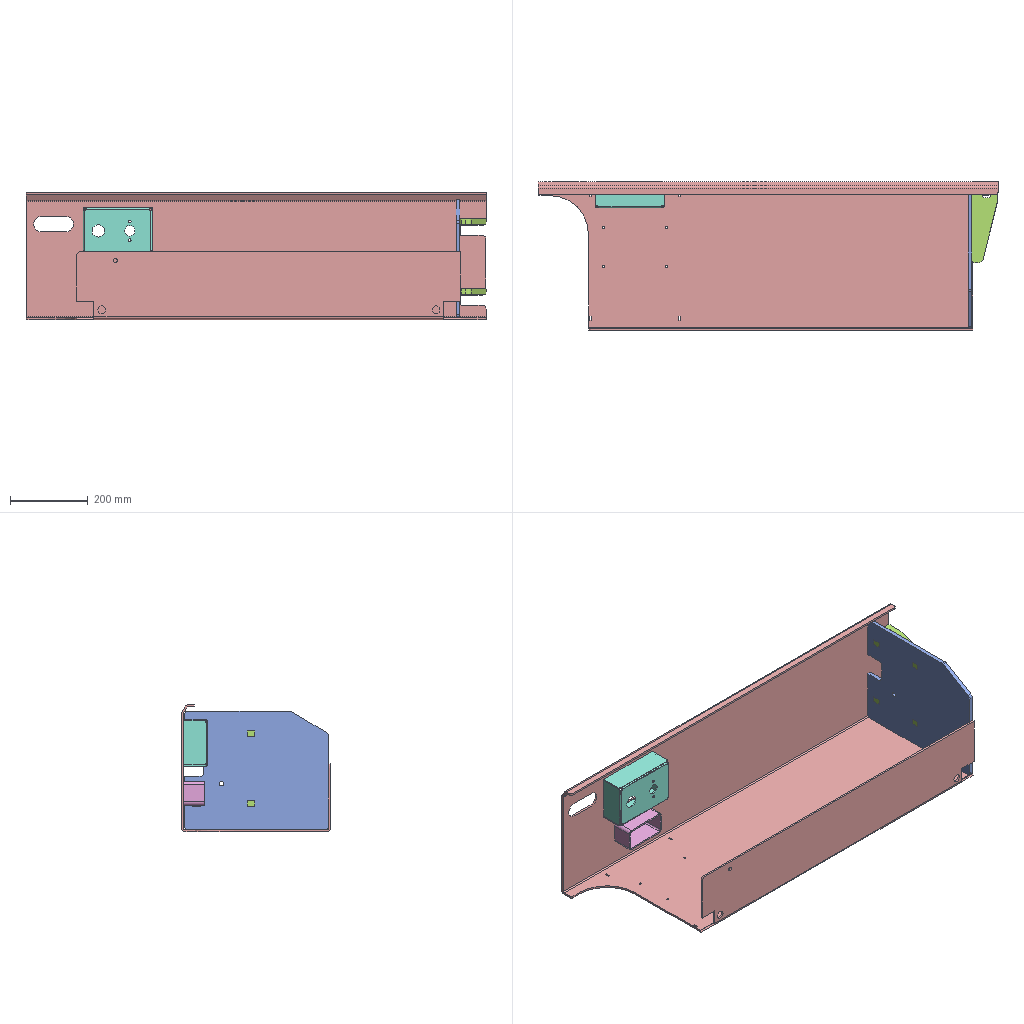Assembly | SolidWorks | 5 different items | 6 placed | box 1184 x 382 x 328 mm
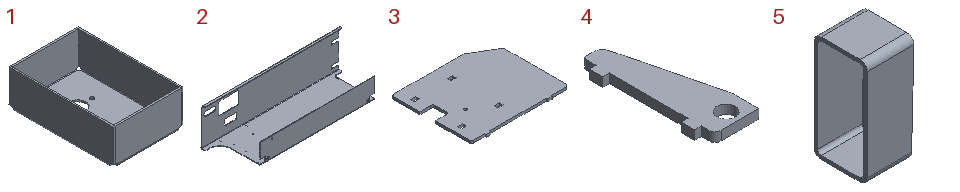Parts list (item | quantity | size | volume | features):
1 | x1 | 119 x 178 x 61.873 mm | 159219 mm3 | features Extrusion 1, FlatPattern 1, SM3dBend 1, SheetMetal 1, SolidToSheetMetal 1
2 | x1 | 1184 x 382 x 327.509 mm | 4582934 mm3 | features SM3dBend 3, Extrusion 1, FlatPattern 1, SheetMetal 1, SolidToSheetMetal 1
3 | x1 | 370 x 310 x 10 mm | 1059963 mm3 | features Extrusion 1
4 | x2 | 76.998 x 201 x 14 mm | 139252 mm3 | features Extrusion 1
5 | x1 | 53 x 60 x 120 mm | 68742 mm3 | features ICE 1, WeldMemberFeat 1, WeldmentFeature 1
Mates (type | each side: item.copy, entity, surface, feature):
Coincident | 2.1 face plane Convert Entities1 | 3.1 face plane Boss-Extrude1 | 3 times
Coincident | 3.1 face plane Boss-Extrude1 | 4.1 face plane Boss-Extrude2 | 3 times
Coincident | 3.1 face plane Boss-Extrude1 | 4.2 face plane Boss-Extrude2 | 3 times
Coincident | 2.1 face plane Convert Entities1 | 5.1 face plane GB/6728-1986 rectangular hollow section 120 X 60 X 4(1) | 3 times
Coincident | 2.1 face plane Convert Entities1 | 1.1 face plane Convert Entities1 | 3 times